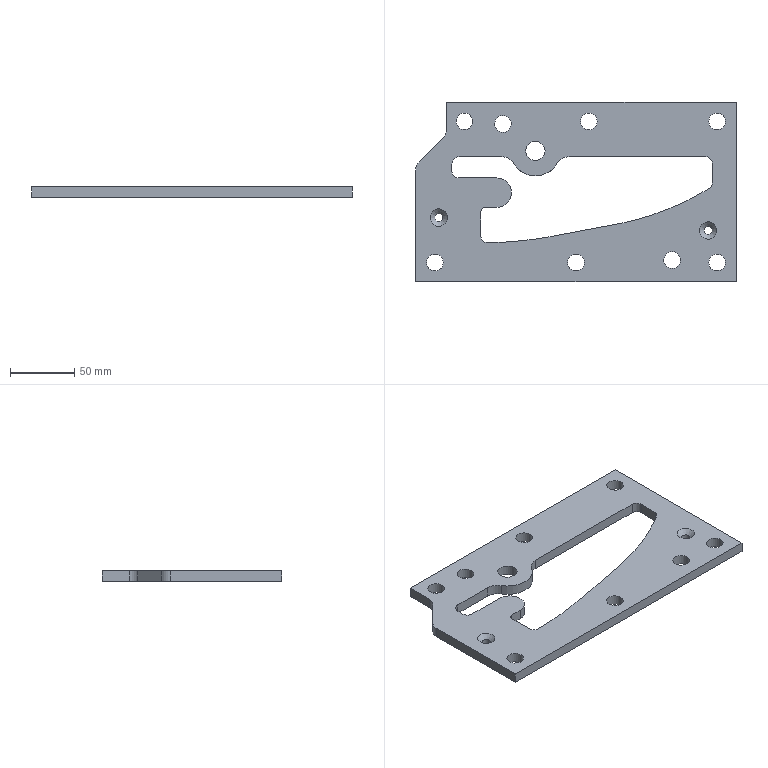Part | STEP file | gslz 2016.10.28-13_id762_x_t | 1 solid | 53 faces | box 250 x 140 x 8 mm | volume 190473 mm3 | plane 26 | cylinder 25 | cone 2 | commonest cylinder face diameters 13 x8 10 x4 6.5 x2 18 x2 22 x2 7 x1